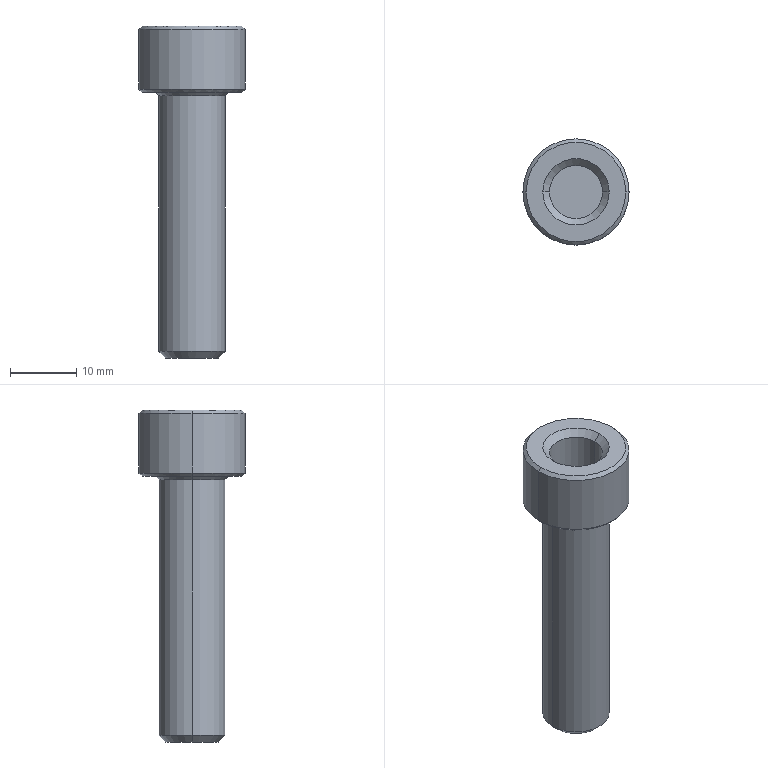Part | STEP file | fBY02F02M-00-11A | 1 solid | 20 faces | box 16 x 16 x 50 mm | volume 4764 mm3 | cone 10 | cylinder 6 | plane 4 | commonest cylinder face diameters 8 x2 10 x2 16 x2
STEP:
#1=CARTESIAN_POINT('',(0.,0.,0.));
#2=DIRECTION('',(0.,0.,1.));
#3=DIRECTION('',(1.,0.,0.));
#4=AXIS2_PLACEMENT_3D('',#1,#2,#3);
#5=CARTESIAN_POINT('',(-5.,0.,39.5));
#6=VERTEX_POINT('',#5);
#7=CARTESIAN_POINT('',(5.,0.,39.5));
#8=VERTEX_POINT('',#7);
#9=CARTESIAN_POINT('',(0.,0.,39.5));
#10=DIRECTION('',(0.,0.,-1.));
#11=DIRECTION('',(-1.,0.,0.));
#12=AXIS2_PLACEMENT_3D('',#9,#10,#11);
#13=CIRCLE('',#12,5.);
#14=CARTESIAN_POINT('',(0.,0.,40.));
#15=DIRECTION('',(0.,0.,-1.));
#16=DIRECTION('',(-1.,0.,0.));
#17=AXIS2_PLACEMENT_3D('',#14,#15,#16);
#18=CYLINDRICAL_SURFACE('',#17,5.);
#19=CARTESIAN_POINT('',(0.,0.5));
#20=DIRECTION('',(1.,0.));
#21=VECTOR('',#20,1.);
#22=LINE('',#19,#21);
#23=(GEOMETRIC_REPRESENTATION_CONTEXT(2)PARAMETRIC_REPRESENTATION_CONTEXT()REPRESENTATION_CONTEXT('',''));
#24=DEFINITIONAL_REPRESENTATION('',(#22),#23);
#25=PCURVE('',#18,#24);
#26=CARTESIAN_POINT('',(0.,0.,40.));
#27=DIRECTION('',(0.,0.,1.));
#28=DIRECTION('',(1.,0.,0.));
#29=AXIS2_PLACEMENT_3D('',#26,#27,#28);
#30=CONICAL_SURFACE('',#29,5.5,0.7854);
#31=CARTESIAN_POINT('',(3.142,-0.5));
#32=DIRECTION('',(-1.,0.));
#33=VECTOR('',#32,1.);
#34=LINE('',#31,#33);
#35=(GEOMETRIC_REPRESENTATION_CONTEXT(2)PARAMETRIC_REPRESENTATION_CONTEXT()REPRESENTATION_CONTEXT('',''));
#36=DEFINITIONAL_REPRESENTATION('',(#34),#35);
#37=PCURVE('',#30,#36);
#38=SURFACE_CURVE('',#13,(#25,#37),.PCURVE_S1.);
#39=EDGE_CURVE('',#6,#8,#38,.T.);
#40=ORIENTED_EDGE('',*,*,#39,.T.);
#41=CARTESIAN_POINT('',(5.,0.,1.));
#42=VERTEX_POINT('',#41);
#43=CARTESIAN_POINT('',(5.,0.,40.));
#44=DIRECTION('',(0.,0.,-1.));
#45=VECTOR('',#44,1.);
#46=LINE('',#43,#45);
#47=CARTESIAN_POINT('',(3.142,0.));
#48=DIRECTION('',(0.,1.));
#49=VECTOR('',#48,1.);
#50=LINE('',#47,#49);
#51=(GEOMETRIC_REPRESENTATION_CONTEXT(2)PARAMETRIC_REPRESENTATION_CONTEXT()REPRESENTATION_CONTEXT('',''));
#52=DEFINITIONAL_REPRESENTATION('',(#50),#51);
#53=PCURVE('',#18,#52);
#54=CARTESIAN_POINT('',(0.,0.,40.));
#55=DIRECTION('',(0.,0.,-1.));
#56=DIRECTION('',(-1.,0.,0.));
#57=AXIS2_PLACEMENT_3D('',#54,#55,#56);
#58=CYLINDRICAL_SURFACE('',#57,5.);
#59=CARTESIAN_POINT('',(3.142,0.));
#60=DIRECTION('',(0.,1.));
#61=VECTOR('',#60,1.);
#62=LINE('',#59,#61);
#63=(GEOMETRIC_REPRESENTATION_CONTEXT(2)PARAMETRIC_REPRESENTATION_CONTEXT()REPRESENTATION_CONTEXT('',''));
#64=DEFINITIONAL_REPRESENTATION('',(#62),#63);
#65=PCURVE('',#58,#64);
#66=SURFACE_CURVE('',#46,(#53,#65),.PCURVE_S1.);
#67=EDGE_CURVE('',#8,#42,#66,.T.);
#68=ORIENTED_EDGE('',*,*,#67,.T.);
#69=CARTESIAN_POINT('',(-5.,0.,1.));
#70=VERTEX_POINT('',#69);
#71=CARTESIAN_POINT('',(0.,0.,1.));
#72=DIRECTION('',(0.,0.,1.));
#73=DIRECTION('',(-1.,0.,0.));
#74=AXIS2_PLACEMENT_3D('',#71,#72,#73);
#75=CIRCLE('',#74,5.);
#76=CARTESIAN_POINT('',(6.283,39.));
#77=DIRECTION('',(-1.,0.));
#78=VECTOR('',#77,1.);
#79=LINE('',#76,#78);
#80=(GEOMETRIC_REPRESENTATION_CONTEXT(2)PARAMETRIC_REPRESENTATION_CONTEXT()REPRESENTATION_CONTEXT('',''));
#81=DEFINITIONAL_REPRESENTATION('',(#79),#80);
#82=PCURVE('',#18,#81);
#83=CARTESIAN_POINT('',(0.,0.,1.));
#84=DIRECTION('',(0.,0.,1.));
#85=DIRECTION('',(1.,0.,0.));
#86=AXIS2_PLACEMENT_3D('',#83,#84,#85);
#87=CONICAL_SURFACE('',#86,5.,0.7854);
#88=CARTESIAN_POINT('',(-3.142,0.));
#89=DIRECTION('',(1.,0.));
#90=VECTOR('',#89,1.);
#91=LINE('',#88,#90);
#92=(GEOMETRIC_REPRESENTATION_CONTEXT(2)PARAMETRIC_REPRESENTATION_CONTEXT()REPRESENTATION_CONTEXT('',''));
#93=DEFINITIONAL_REPRESENTATION('',(#91),#92);
#94=PCURVE('',#87,#93);
#95=SURFACE_CURVE('',#75,(#82,#94),.PCURVE_S1.);
#96=EDGE_CURVE('',#42,#70,#95,.T.);
#97=ORIENTED_EDGE('',*,*,#96,.T.);
#98=CARTESIAN_POINT('',(-5.,0.,40.));
#99=DIRECTION('',(0.,0.,-1.));
#100=VECTOR('',#99,1.);
#101=LINE('',#98,#100);
#102=CARTESIAN_POINT('',(0.,0.));
#103=DIRECTION('',(0.,1.));
#104=VECTOR('',#103,1.);
#105=LINE('',#102,#104);
#106=(GEOMETRIC_REPRESENTATION_CONTEXT(2)PARAMETRIC_REPRESENTATION_CONTEXT()REPRESENTATION_CONTEXT('',''));
#107=DEFINITIONAL_REPRESENTATION('',(#105),#106);
#108=PCURVE('',#18,#107);
#109=CARTESIAN_POINT('',(6.283,0.));
#110=DIRECTION('',(0.,1.));
#111=VECTOR('',#110,1.);
#112=LINE('',#109,#111);
#113=(GEOMETRIC_REPRESENTATION_CONTEXT(2)PARAMETRIC_REPRESENTATION_CONTEXT()REPRESENTATION_CONTEXT('',''));
#114=DEFINITIONAL_REPRESENTATION('',(#112),#113);
#115=PCURVE('',#58,#114);
#116=SURFACE_CURVE('',#101,(#108,#115),.PCURVE_S1.);
#117=EDGE_CURVE('',#6,#70,#116,.T.);
#118=ORIENTED_EDGE('',*,*,#117,.F.);
#119=EDGE_LOOP('',(#40,#68,#97,#118));
#120=FACE_BOUND('',#119,.T.);
#121=ADVANCED_FACE('',(#120),#18,.T.);
#122=CARTESIAN_POINT('',(4.,0.,0.));
#123=VERTEX_POINT('',#122);
#124=CARTESIAN_POINT('',(-4.,0.,0.));
#125=VERTEX_POINT('',#124);
#126=CARTESIAN_POINT('',(0.,0.,0.));
#127=DIRECTION('',(0.,0.,1.));
#128=DIRECTION('',(1.,0.,0.));
#129=AXIS2_PLACEMENT_3D('',#126,#127,#128);
#130=CIRCLE('',#129,4.);
#131=CARTESIAN_POINT('',(0.,-1.));
#132=DIRECTION('',(1.,0.));
#133=VECTOR('',#132,1.);
#134=LINE('',#131,#133);
#135=(GEOMETRIC_REPRESENTATION_CONTEXT(2)PARAMETRIC_REPRESENTATION_CONTEXT()REPRESENTATION_CONTEXT('',''));
#136=DEFINITIONAL_REPRESENTATION('',(#134),#135);
#137=PCURVE('',#87,#136);
#138=CARTESIAN_POINT('',(0.,0.,0.));
#139=DIRECTION('',(0.,0.,1.));
#140=DIRECTION('',(1.,0.,0.));
#141=AXIS2_PLACEMENT_3D('',#138,#139,#140);
#142=PLANE('',#141);
#143=CARTESIAN_POINT('',(0.,0.));
#144=DIRECTION('',(1.,0.));
#145=AXIS2_PLACEMENT_2D('',#143,#144);
#146=CIRCLE('',#145,4.);
#147=(GEOMETRIC_REPRESENTATION_CONTEXT(2)PARAMETRIC_REPRESENTATION_CONTEXT()REPRESENTATION_CONTEXT('',''));
#148=DEFINITIONAL_REPRESENTATION('',(#146),#147);
#149=PCURVE('',#142,#148);
#150=SURFACE_CURVE('',#130,(#137,#149),.PCURVE_S1.);
#151=EDGE_CURVE('',#123,#125,#150,.T.);
#152=ORIENTED_EDGE('',*,*,#151,.T.);
#153=CARTESIAN_POINT('',(-5.,0.,1.));
#154=DIRECTION('',(-0.7071,0.,0.7071));
#155=VECTOR('',#154,1.);
#156=LINE('',#153,#155);
#157=CARTESIAN_POINT('',(3.142,0.));
#158=DIRECTION('',(0.,1.));
#159=VECTOR('',#158,1.);
#160=LINE('',#157,#159);
#161=(GEOMETRIC_REPRESENTATION_CONTEXT(2)PARAMETRIC_REPRESENTATION_CONTEXT()REPRESENTATION_CONTEXT('',''));
#162=DEFINITIONAL_REPRESENTATION('',(#160),#161);
#163=PCURVE('',#87,#162);
#164=CARTESIAN_POINT('',(0.,0.,1.));
#165=DIRECTION('',(0.,0.,1.));
#166=DIRECTION('',(1.,0.,0.));
#167=AXIS2_PLACEMENT_3D('',#164,#165,#166);
#168=CONICAL_SURFACE('',#167,5.,0.7854);
#169=CARTESIAN_POINT('',(3.142,0.));
#170=DIRECTION('',(0.,1.));
#171=VECTOR('',#170,1.);
#172=LINE('',#169,#171);
#173=(GEOMETRIC_REPRESENTATION_CONTEXT(2)PARAMETRIC_REPRESENTATION_CONTEXT()REPRESENTATION_CONTEXT('',''));
#174=DEFINITIONAL_REPRESENTATION('',(#172),#173);
#175=PCURVE('',#168,#174);
#176=SURFACE_CURVE('',#156,(#163,#175),.PCURVE_S1.);
#177=EDGE_CURVE('',#125,#70,#176,.T.);
#178=ORIENTED_EDGE('',*,*,#177,.T.);
#179=ORIENTED_EDGE('',*,*,#96,.F.);
#180=CARTESIAN_POINT('',(5.,0.,1.));
#181=DIRECTION('',(0.7071,0.,0.7071));
#182=VECTOR('',#181,1.);
#183=LINE('',#180,#182);
#184=CARTESIAN_POINT('',(0.,0.));
#185=DIRECTION('',(0.,1.));
#186=VECTOR('',#185,1.);
#187=LINE('',#184,#186);
#188=(GEOMETRIC_REPRESENTATION_CONTEXT(2)PARAMETRIC_REPRESENTATION_CONTEXT()REPRESENTATION_CONTEXT('',''));
#189=DEFINITIONAL_REPRESENTATION('',(#187),#188);
#190=PCURVE('',#87,#189);
#191=CARTESIAN_POINT('',(6.283,0.));
#192=DIRECTION('',(0.,1.));
#193=VECTOR('',#192,1.);
#194=LINE('',#191,#193);
#195=(GEOMETRIC_REPRESENTATION_CONTEXT(2)PARAMETRIC_REPRESENTATION_CONTEXT()REPRESENTATION_CONTEXT('',''));
#196=DEFINITIONAL_REPRESENTATION('',(#194),#195);
#197=PCURVE('',#168,#196);
#198=SURFACE_CURVE('',#183,(#190,#197),.PCURVE_S1.);
#199=EDGE_CURVE('',#123,#42,#198,.T.);
#200=ORIENTED_EDGE('',*,*,#199,.F.);
#201=EDGE_LOOP('',(#152,#178,#179,#200));
#202=FACE_BOUND('',#201,.T.);
#203=ADVANCED_FACE('',(#202),#87,.T.);
#204=ORIENTED_EDGE('',*,*,#39,.F.);
#205=CARTESIAN_POINT('',(-5.5,0.,40.));
#206=VERTEX_POINT('',#205);
#207=CARTESIAN_POINT('',(-5.5,0.,40.));
#208=DIRECTION('',(-0.7071,0.,0.7071));
#209=VECTOR('',#208,1.);
#210=LINE('',#207,#209);
#211=CARTESIAN_POINT('',(3.142,0.));
#212=DIRECTION('',(0.,1.));
#213=VECTOR('',#212,1.);
#214=LINE('',#211,#213);
#215=(GEOMETRIC_REPRESENTATION_CONTEXT(2)PARAMETRIC_REPRESENTATION_CONTEXT()REPRESENTATION_CONTEXT('',''));
#216=DEFINITIONAL_REPRESENTATION('',(#214),#215);
#217=PCURVE('',#30,#216);
#218=CARTESIAN_POINT('',(0.,0.,40.));
#219=DIRECTION('',(0.,0.,1.));
#220=DIRECTION('',(1.,0.,0.));
#221=AXIS2_PLACEMENT_3D('',#218,#219,#220);
#222=CONICAL_SURFACE('',#221,5.5,0.7854);
#223=CARTESIAN_POINT('',(3.142,0.));
#224=DIRECTION('',(0.,1.));
#225=VECTOR('',#224,1.);
#226=LINE('',#223,#225);
#227=(GEOMETRIC_REPRESENTATION_CONTEXT(2)PARAMETRIC_REPRESENTATION_CONTEXT()REPRESENTATION_CONTEXT('',''));
#228=DEFINITIONAL_REPRESENTATION('',(#226),#227);
#229=PCURVE('',#222,#228);
#230=SURFACE_CURVE('',#210,(#217,#229),.PCURVE_S1.);
#231=EDGE_CURVE('',#6,#206,#230,.T.);
#232=ORIENTED_EDGE('',*,*,#231,.T.);
#233=CARTESIAN_POINT('',(5.5,0.,40.));
#234=VERTEX_POINT('',#233);
#235=CARTESIAN_POINT('',(0.,0.,40.));
#236=DIRECTION('',(0.,0.,-1.));
#237=DIRECTION('',(1.,0.,0.));
#238=AXIS2_PLACEMENT_3D('',#235,#236,#237);
#239=CIRCLE('',#238,5.5);
#240=CARTESIAN_POINT('',(6.283,0.));
#241=DIRECTION('',(-1.,0.));
#242=VECTOR('',#241,1.);
#243=LINE('',#240,#242);
#244=(GEOMETRIC_REPRESENTATION_CONTEXT(2)PARAMETRIC_REPRESENTATION_CONTEXT()REPRESENTATION_CONTEXT('',''));
#245=DEFINITIONAL_REPRESENTATION('',(#243),#244);
#246=PCURVE('',#30,#245);
#247=CARTESIAN_POINT('',(0.,0.,40.));
#248=DIRECTION('',(0.,0.,1.));
#249=DIRECTION('',(1.,0.,0.));
#250=AXIS2_PLACEMENT_3D('',#247,#248,#249);
#251=PLANE('',#250);
#252=CARTESIAN_POINT('',(5.5,0.));
#253=CARTESIAN_POINT('',(5.5,-9.526));
#254=CARTESIAN_POINT('',(-2.75,-4.763));
#255=CARTESIAN_POINT('',(-11.,0.));
#256=CARTESIAN_POINT('',(-2.75,4.763));
#257=CARTESIAN_POINT('',(5.5,9.526));
#258=CARTESIAN_POINT('',(5.5,0.));
#259=(BOUNDED_CURVE()B_SPLINE_CURVE(2,(#252,#253,#254,#255,#256,#257,#258),.UNSPECIFIED.,.T.,.F.)B_SPLINE_CURVE_WITH_KNOTS((1,2,2,2,2,1),(-2.094,0.,2.094,4.189,6.283,8.378),.UNSPECIFIED.)CURVE()GEOMETRIC_REPRESENTATION_ITEM()RATIONAL_B_SPLINE_CURVE((1.,0.5,1.,0.5,1.,0.5,1.))REPRESENTATION_ITEM(''));
#260=(GEOMETRIC_REPRESENTATION_CONTEXT(2)PARAMETRIC_REPRESENTATION_CONTEXT()REPRESENTATION_CONTEXT('',''));
#261=DEFINITIONAL_REPRESENTATION('',(#259),#260);
#262=PCURVE('',#251,#261);
#263=SURFACE_CURVE('',#239,(#246,#262),.PCURVE_S1.);
#264=EDGE_CURVE('',#206,#234,#263,.T.);
#265=ORIENTED_EDGE('',*,*,#264,.T.);
#266=CARTESIAN_POINT('',(5.5,0.,40.));
#267=DIRECTION('',(0.7071,0.,0.7071));
#268=VECTOR('',#267,1.);
#269=LINE('',#266,#268);
#270=CARTESIAN_POINT('',(0.,0.));
#271=DIRECTION('',(0.,1.));
#272=VECTOR('',#271,1.);
#273=LINE('',#270,#272);
#274=(GEOMETRIC_REPRESENTATION_CONTEXT(2)PARAMETRIC_REPRESENTATION_CONTEXT()REPRESENTATION_CONTEXT('',''));
#275=DEFINITIONAL_REPRESENTATION('',(#273),#274);
#276=PCURVE('',#30,#275);
#277=CARTESIAN_POINT('',(6.283,0.));
#278=DIRECTION('',(0.,1.));
#279=VECTOR('',#278,1.);
#280=LINE('',#277,#279);
#281=(GEOMETRIC_REPRESENTATION_CONTEXT(2)PARAMETRIC_REPRESENTATION_CONTEXT()REPRESENTATION_CONTEXT('',''));
#282=DEFINITIONAL_REPRESENTATION('',(#280),#281);
#283=PCURVE('',#222,#282);
#284=SURFACE_CURVE('',#269,(#276,#283),.PCURVE_S1.);
#285=EDGE_CURVE('',#8,#234,#284,.T.);
#286=ORIENTED_EDGE('',*,*,#285,.F.);
#287=EDGE_LOOP('',(#204,#232,#265,#286));
#288=FACE_BOUND('',#287,.T.);
#289=ADVANCED_FACE('',(#288),#30,.T.);
#290=CARTESIAN_POINT('',(7.5,0.,40.));
#291=VERTEX_POINT('',#290);
#292=CARTESIAN_POINT('',(-7.5,0.,40.));
#293=VERTEX_POINT('',#292);
#294=CARTESIAN_POINT('',(0.,0.,40.));
#295=DIRECTION('',(0.,0.,1.));
#296=DIRECTION('',(1.,0.,0.));
#297=AXIS2_PLACEMENT_3D('',#294,#295,#296);
#298=CIRCLE('',#297,7.5);
#299=CARTESIAN_POINT('',(0.,0.,40.5));
#300=DIRECTION('',(0.,0.,1.));
#301=DIRECTION('',(1.,0.,0.));
#302=AXIS2_PLACEMENT_3D('',#299,#300,#301);
#303=CONICAL_SURFACE('',#302,8.,0.7854);
#304=CARTESIAN_POINT('',(0.,-0.5));
#305=DIRECTION('',(1.,0.));
#306=VECTOR('',#305,1.);
#307=LINE('',#304,#306);
#308=(GEOMETRIC_REPRESENTATION_CONTEXT(2)PARAMETRIC_REPRESENTATION_CONTEXT()REPRESENTATION_CONTEXT('',''));
#309=DEFINITIONAL_REPRESENTATION('',(#307),#308);
#310=PCURVE('',#303,#309);
#311=CARTESIAN_POINT('',(0.,0.));
#312=DIRECTION('',(1.,0.));
#313=AXIS2_PLACEMENT_2D('',#311,#312);
#314=CIRCLE('',#313,7.5);
#315=(GEOMETRIC_REPRESENTATION_CONTEXT(2)PARAMETRIC_REPRESENTATION_CONTEXT()REPRESENTATION_CONTEXT('',''));
#316=DEFINITIONAL_REPRESENTATION('',(#314),#315);
#317=PCURVE('',#251,#316);
#318=SURFACE_CURVE('',#298,(#310,#317),.PCURVE_S1.);
#319=EDGE_CURVE('',#291,#293,#318,.T.);
#320=ORIENTED_EDGE('',*,*,#319,.T.);
#321=CARTESIAN_POINT('',(-8.,0.,40.5));
#322=VERTEX_POINT('',#321);
#323=CARTESIAN_POINT('',(-8.,0.,40.5));
#324=DIRECTION('',(-0.7071,0.,0.7071));
#325=VECTOR('',#324,1.);
#326=LINE('',#323,#325);
#327=CARTESIAN_POINT('',(3.142,0.));
#328=DIRECTION('',(0.,1.));
#329=VECTOR('',#328,1.);
#330=LINE('',#327,#329);
#331=(GEOMETRIC_REPRESENTATION_CONTEXT(2)PARAMETRIC_REPRESENTATION_CONTEXT()REPRESENTATION_CONTEXT('',''));
#332=DEFINITIONAL_REPRESENTATION('',(#330),#331);
#333=PCURVE('',#303,#332);
#334=CARTESIAN_POINT('',(0.,0.,40.5));
#335=DIRECTION('',(0.,0.,1.));
#336=DIRECTION('',(1.,0.,0.));
#337=AXIS2_PLACEMENT_3D('',#334,#335,#336);
#338=CONICAL_SURFACE('',#337,8.,0.7854);
#339=CARTESIAN_POINT('',(3.142,0.));
#340=DIRECTION('',(0.,1.));
#341=VECTOR('',#340,1.);
#342=LINE('',#339,#341);
#343=(GEOMETRIC_REPRESENTATION_CONTEXT(2)PARAMETRIC_REPRESENTATION_CONTEXT()REPRESENTATION_CONTEXT('',''));
#344=DEFINITIONAL_REPRESENTATION('',(#342),#343);
#345=PCURVE('',#338,#344);
#346=SURFACE_CURVE('',#326,(#333,#345),.PCURVE_S1.);
#347=EDGE_CURVE('',#293,#322,#346,.T.);
#348=ORIENTED_EDGE('',*,*,#347,.T.);
#349=CARTESIAN_POINT('',(8.,0.,40.5));
#350=VERTEX_POINT('',#349);
#351=CARTESIAN_POINT('',(0.,0.,40.5));
#352=DIRECTION('',(0.,0.,-1.));
#353=DIRECTION('',(1.,0.,0.));
#354=AXIS2_PLACEMENT_3D('',#351,#352,#353);
#355=CIRCLE('',#354,8.);
#356=CARTESIAN_POINT('',(6.283,0.));
#357=DIRECTION('',(-1.,0.));
#358=VECTOR('',#357,1.);
#359=LINE('',#356,#358);
#360=(GEOMETRIC_REPRESENTATION_CONTEXT(2)PARAMETRIC_REPRESENTATION_CONTEXT()REPRESENTATION_CONTEXT('',''));
#361=DEFINITIONAL_REPRESENTATION('',(#359),#360);
#362=PCURVE('',#303,#361);
#363=CARTESIAN_POINT('',(0.,0.,50.));
#364=DIRECTION('',(0.,0.,-1.));
#365=DIRECTION('',(-1.,0.,0.));
#366=AXIS2_PLACEMENT_3D('',#363,#364,#365);
#367=CYLINDRICAL_SURFACE('',#366,8.);
#368=CARTESIAN_POINT('',(-3.142,9.5));
#369=DIRECTION('',(1.,0.));
#370=VECTOR('',#369,1.);
#371=LINE('',#368,#370);
#372=(GEOMETRIC_REPRESENTATION_CONTEXT(2)PARAMETRIC_REPRESENTATION_CONTEXT()REPRESENTATION_CONTEXT('',''));
#373=DEFINITIONAL_REPRESENTATION('',(#371),#372);
#374=PCURVE('',#367,#373);
#375=SURFACE_CURVE('',#355,(#362,#374),.PCURVE_S1.);
#376=EDGE_CURVE('',#322,#350,#375,.T.);
#377=ORIENTED_EDGE('',*,*,#376,.T.);
#378=CARTESIAN_POINT('',(8.,0.,40.5));
#379=DIRECTION('',(0.7071,0.,0.7071));
#380=VECTOR('',#379,1.);
#381=LINE('',#378,#380);
#382=CARTESIAN_POINT('',(0.,0.));
#383=DIRECTION('',(0.,1.));
#384=VECTOR('',#383,1.);
#385=LINE('',#382,#384);
#386=(GEOMETRIC_REPRESENTATION_CONTEXT(2)PARAMETRIC_REPRESENTATION_CONTEXT()REPRESENTATION_CONTEXT('',''));
#387=DEFINITIONAL_REPRESENTATION('',(#385),#386);
#388=PCURVE('',#303,#387);
#389=CARTESIAN_POINT('',(6.283,0.));
#390=DIRECTION('',(0.,1.));
#391=VECTOR('',#390,1.);
#392=LINE('',#389,#391);
#393=(GEOMETRIC_REPRESENTATION_CONTEXT(2)PARAMETRIC_REPRESENTATION_CONTEXT()REPRESENTATION_CONTEXT('',''));
#394=DEFINITIONAL_REPRESENTATION('',(#392),#393);
#395=PCURVE('',#338,#394);
#396=SURFACE_CURVE('',#381,(#388,#395),.PCURVE_S1.);
#397=EDGE_CURVE('',#291,#350,#396,.T.);
#398=ORIENTED_EDGE('',*,*,#397,.F.);
#399=EDGE_LOOP('',(#320,#348,#377,#398));
#400=FACE_BOUND('',#399,.T.);
#401=ADVANCED_FACE('',(#400),#303,.T.);
#402=CARTESIAN_POINT('',(-8.,0.,49.5));
#403=VERTEX_POINT('',#402);
#404=CARTESIAN_POINT('',(8.,0.,49.5));
#405=VERTEX_POINT('',#404);
#406=CARTESIAN_POINT('',(0.,0.,49.5));
#407=DIRECTION('',(0.,0.,-1.));
#408=DIRECTION('',(-1.,0.,0.));
#409=AXIS2_PLACEMENT_3D('',#406,#407,#408);
#410=CIRCLE('',#409,8.);
#411=CARTESIAN_POINT('',(0.,0.5));
#412=DIRECTION('',(1.,0.));
#413=VECTOR('',#412,1.);
#414=LINE('',#411,#413);
#415=(GEOMETRIC_REPRESENTATION_CONTEXT(2)PARAMETRIC_REPRESENTATION_CONTEXT()REPRESENTATION_CONTEXT('',''));
#416=DEFINITIONAL_REPRESENTATION('',(#414),#415);
#417=PCURVE('',#367,#416);
#418=CARTESIAN_POINT('',(0.,0.,49.5));
#419=DIRECTION('',(0.,0.,-1.));
#420=DIRECTION('',(-1.,0.,0.));
#421=AXIS2_PLACEMENT_3D('',#418,#419,#420);
#422=CONICAL_SURFACE('',#421,8.,0.7854);
#423=CARTESIAN_POINT('',(0.,0.));
#424=DIRECTION('',(1.,0.));
#425=VECTOR('',#424,1.);
#426=LINE('',#423,#425);
#427=(GEOMETRIC_REPRESENTATION_CONTEXT(2)PARAMETRIC_REPRESENTATION_CONTEXT()REPRESENTATION_CONTEXT('',''));
#428=DEFINITIONAL_REPRESENTATION('',(#426),#427);
#429=PCURVE('',#422,#428);
#430=SURFACE_CURVE('',#410,(#417,#429),.PCURVE_S1.);
#431=EDGE_CURVE('',#403,#405,#430,.T.);
#432=ORIENTED_EDGE('',*,*,#431,.T.);
#433=CARTESIAN_POINT('',(8.,0.,50.));
#434=DIRECTION('',(0.,0.,-1.));
#435=VECTOR('',#434,1.);
#436=LINE('',#433,#435);
#437=CARTESIAN_POINT('',(3.142,0.));
#438=DIRECTION('',(0.,1.));
#439=VECTOR('',#438,1.);
#440=LINE('',#437,#439);
#441=(GEOMETRIC_REPRESENTATION_CONTEXT(2)PARAMETRIC_REPRESENTATION_CONTEXT()REPRESENTATION_CONTEXT('',''));
#442=DEFINITIONAL_REPRESENTATION('',(#440),#441);
#443=PCURVE('',#367,#442);
#444=CARTESIAN_POINT('',(0.,0.,50.));
#445=DIRECTION('',(0.,0.,-1.));
#446=DIRECTION('',(-1.,0.,0.));
#447=AXIS2_PLACEMENT_3D('',#444,#445,#446);
#448=CYLINDRICAL_SURFACE('',#447,8.);
#449=CARTESIAN_POINT('',(3.142,0.));
#450=DIRECTION('',(0.,1.));
#451=VECTOR('',#450,1.);
#452=LINE('',#449,#451);
#453=(GEOMETRIC_REPRESENTATION_CONTEXT(2)PARAMETRIC_REPRESENTATION_CONTEXT()REPRESENTATION_CONTEXT('',''));
#454=DEFINITIONAL_REPRESENTATION('',(#452),#453);
#455=PCURVE('',#448,#454);
#456=SURFACE_CURVE('',#436,(#443,#455),.PCURVE_S1.);
#457=EDGE_CURVE('',#405,#350,#456,.T.);
#458=ORIENTED_EDGE('',*,*,#457,.T.);
#459=ORIENTED_EDGE('',*,*,#376,.F.);
#460=CARTESIAN_POINT('',(-8.,0.,50.));
#461=DIRECTION('',(0.,0.,-1.));
#462=VECTOR('',#461,1.);
#463=LINE('',#460,#462);
#464=CARTESIAN_POINT('',(0.,0.));
#465=DIRECTION('',(0.,1.));
#466=VECTOR('',#465,1.);
#467=LINE('',#464,#466);
#468=(GEOMETRIC_REPRESENTATION_CONTEXT(2)PARAMETRIC_REPRESENTATION_CONTEXT()REPRESENTATION_CONTEXT('',''));
#469=DEFINITIONAL_REPRESENTATION('',(#467),#468);
#470=PCURVE('',#367,#469);
#471=CARTESIAN_POINT('',(6.283,0.));
#472=DIRECTION('',(0.,1.));
#473=VECTOR('',#472,1.);
#474=LINE('',#471,#473);
#475=(GEOMETRIC_REPRESENTATION_CONTEXT(2)PARAMETRIC_REPRESENTATION_CONTEXT()REPRESENTATION_CONTEXT('',''));
#476=DEFINITIONAL_REPRESENTATION('',(#474),#475);
#477=PCURVE('',#448,#476);
#478=SURFACE_CURVE('',#463,(#470,#477),.PCURVE_S1.);
#479=EDGE_CURVE('',#403,#322,#478,.T.);
#480=ORIENTED_EDGE('',*,*,#479,.F.);
#481=EDGE_LOOP('',(#432,#458,#459,#480));
#482=FACE_BOUND('',#481,.T.);
#483=ADVANCED_FACE('',(#482),#367,.T.);
#484=CARTESIAN_POINT('',(-7.5,0.,50.));
#485=VERTEX_POINT('',#484);
#486=CARTESIAN_POINT('',(7.5,0.,50.));
#487=VERTEX_POINT('',#486);
#488=CARTESIAN_POINT('',(0.,0.,50.));
#489=DIRECTION('',(0.,0.,-1.));
#490=DIRECTION('',(-1.,0.,0.));
#491=AXIS2_PLACEMENT_3D('',#488,#489,#490);
#492=CIRCLE('',#491,7.5);
#493=CARTESIAN_POINT('',(0.,-0.5));
#494=DIRECTION('',(1.,0.));
#495=VECTOR('',#494,1.);
#496=LINE('',#493,#495);
#497=(GEOMETRIC_REPRESENTATION_CONTEXT(2)PARAMETRIC_REPRESENTATION_CONTEXT()REPRESENTATION_CONTEXT('',''));
#498=DEFINITIONAL_REPRESENTATION('',(#496),#497);
#499=PCURVE('',#422,#498);
#500=CARTESIAN_POINT('',(0.,0.,50.));
#501=DIRECTION('',(0.,0.,1.));
#502=DIRECTION('',(1.,0.,0.));
#503=AXIS2_PLACEMENT_3D('',#500,#501,#502);
#504=PLANE('',#503);
#505=CARTESIAN_POINT('',(-7.5,0.));
#506=CARTESIAN_POINT('',(-7.5,12.99));
#507=CARTESIAN_POINT('',(3.75,6.495));
#508=CARTESIAN_POINT('',(15.,0.));
#509=CARTESIAN_POINT('',(3.75,-6.495));
#510=CARTESIAN_POINT('',(-7.5,-12.99));
#511=CARTESIAN_POINT('',(-7.5,0.));
#512=(BOUNDED_CURVE()B_SPLINE_CURVE(2,(#505,#506,#507,#508,#509,#510,#511),.UNSPECIFIED.,.T.,.F.)B_SPLINE_CURVE_WITH_KNOTS((1,2,2,2,2,1),(-2.094,0.,2.094,4.189,6.283,8.378),.UNSPECIFIED.)CURVE()GEOMETRIC_REPRESENTATION_ITEM()RATIONAL_B_SPLINE_CURVE((1.,0.5,1.,0.5,1.,0.5,1.))REPRESENTATION_ITEM(''));
#513=(GEOMETRIC_REPRESENTATION_CONTEXT(2)PARAMETRIC_REPRESENTATION_CONTEXT()REPRESENTATION_CONTEXT('',''));
#514=DEFINITIONAL_REPRESENTATION('',(#512),#513);
#515=PCURVE('',#504,#514);
#516=SURFACE_CURVE('',#492,(#499,#515),.PCURVE_S1.);
#517=EDGE_CURVE('',#485,#487,#516,.T.);
#518=ORIENTED_EDGE('',*,*,#517,.T.);
#519=CARTESIAN_POINT('',(8.,0.,49.5));
#520=DIRECTION('',(0.7071,0.,-0.7071));
#521=VECTOR('',#520,1.);
#522=LINE('',#519,#521);
#523=CARTESIAN_POINT('',(3.142,0.));
#524=DIRECTION('',(0.,1.));
#525=VECTOR('',#524,1.);
#526=LINE('',#523,#525);
#527=(GEOMETRIC_REPRESENTATION_CONTEXT(2)PARAMETRIC_REPRESENTATION_CONTEXT()REPRESENTATION_CONTEXT('',''));
#528=DEFINITIONAL_REPRESENTATION('',(#526),#527);
#529=PCURVE('',#422,#528);
#530=CARTESIAN_POINT('',(0.,0.,49.5));
#531=DIRECTION('',(0.,0.,-1.));
#532=DIRECTION('',(-1.,0.,0.));
#533=AXIS2_PLACEMENT_3D('',#530,#531,#532);
#534=CONICAL_SURFACE('',#533,8.,0.7854);
#535=CARTESIAN_POINT('',(3.142,0.));
#536=DIRECTION('',(0.,1.));
#537=VECTOR('',#536,1.);
#538=LINE('',#535,#537);
#539=(GEOMETRIC_REPRESENTATION_CONTEXT(2)PARAMETRIC_REPRESENTATION_CONTEXT()REPRESENTATION_CONTEXT('',''));
#540=DEFINITIONAL_REPRESENTATION('',(#538),#539);
#541=PCURVE('',#534,#540);
#542=SURFACE_CURVE('',#522,(#529,#541),.PCURVE_S1.);
#543=EDGE_CURVE('',#487,#405,#542,.T.);
#544=ORIENTED_EDGE('',*,*,#543,.T.);
#545=ORIENTED_EDGE('',*,*,#431,.F.);
#546=CARTESIAN_POINT('',(-8.,0.,49.5));
#547=DIRECTION('',(-0.7071,0.,-0.7071));
#548=VECTOR('',#547,1.);
#549=LINE('',#546,#548);
#550=CARTESIAN_POINT('',(0.,0.));
#551=DIRECTION('',(0.,1.));
#552=VECTOR('',#551,1.);
#553=LINE('',#550,#552);
#554=(GEOMETRIC_REPRESENTATION_CONTEXT(2)PARAMETRIC_REPRESENTATION_CONTEXT()REPRESENTATION_CONTEXT('',''));
#555=DEFINITIONAL_REPRESENTATION('',(#553),#554);
#556=PCURVE('',#422,#555);
#557=CARTESIAN_POINT('',(6.283,0.));
#558=DIRECTION('',(0.,1.));
#559=VECTOR('',#558,1.);
#560=LINE('',#557,#559);
#561=(GEOMETRIC_REPRESENTATION_CONTEXT(2)PARAMETRIC_REPRESENTATION_CONTEXT()REPRESENTATION_CONTEXT('',''));
#562=DEFINITIONAL_REPRESENTATION('',(#560),#561);
#563=PCURVE('',#534,#562);
#564=SURFACE_CURVE('',#549,(#556,#563),.PCURVE_S1.);
#565=EDGE_CURVE('',#485,#403,#564,.T.);
#566=ORIENTED_EDGE('',*,*,#565,.F.);
#567=EDGE_LOOP('',(#518,#544,#545,#566));
#568=FACE_BOUND('',#567,.T.);
#569=ADVANCED_FACE('',(#568),#422,.T.);
#570=CARTESIAN_POINT('',(4.,0.,49.));
#571=VERTEX_POINT('',#570);
#572=CARTESIAN_POINT('',(5.,0.,50.));
#573=VERTEX_POINT('',#572);
#574=CARTESIAN_POINT('',(5.,0.,50.));
#575=DIRECTION('',(0.7071,0.,0.7071));
#576=VECTOR('',#575,1.);
#577=LINE('',#574,#576);
#578=CARTESIAN_POINT('',(0.,0.,50.));
#579=DIRECTION('',(0.,0.,1.));
#580=DIRECTION('',(1.,0.,0.));
#581=AXIS2_PLACEMENT_3D('',#578,#579,#580);
#582=CONICAL_SURFACE('',#581,5.,0.7854);
#583=CARTESIAN_POINT('',(6.283,0.));
#584=DIRECTION('',(0.,1.));
#585=VECTOR('',#584,1.);
#586=LINE('',#583,#585);
#587=(GEOMETRIC_REPRESENTATION_CONTEXT(2)PARAMETRIC_REPRESENTATION_CONTEXT()REPRESENTATION_CONTEXT('',''));
#588=DEFINITIONAL_REPRESENTATION('',(#586),#587);
#589=PCURVE('',#582,#588);
#590=CARTESIAN_POINT('',(0.,0.,50.));
#591=DIRECTION('',(0.,0.,1.));
#592=DIRECTION('',(1.,0.,0.));
#593=AXIS2_PLACEMENT_3D('',#590,#591,#592);
#594=CONICAL_SURFACE('',#593,5.,0.7854);
#595=CARTESIAN_POINT('',(0.,0.));
#596=DIRECTION('',(0.,1.));
#597=VECTOR('',#596,1.);
#598=LINE('',#595,#597);
#599=(GEOMETRIC_REPRESENTATION_CONTEXT(2)PARAMETRIC_REPRESENTATION_CONTEXT()REPRESENTATION_CONTEXT('',''));
#600=DEFINITIONAL_REPRESENTATION('',(#598),#599);
#601=PCURVE('',#594,#600);
#602=SURFACE_CURVE('',#577,(#589,#601),.PCURVE_S1.);
#603=EDGE_CURVE('',#571,#573,#602,.T.);
#604=ORIENTED_EDGE('',*,*,#603,.T.);
#605=CARTESIAN_POINT('',(-5.,0.,50.));
#606=VERTEX_POINT('',#605);
#607=CARTESIAN_POINT('',(0.,0.,50.));
#608=DIRECTION('',(0.,0.,-1.));
#609=DIRECTION('',(1.,0.,0.));
#610=AXIS2_PLACEMENT_3D('',#607,#608,#609);
#611=CIRCLE('',#610,5.);
#612=CARTESIAN_POINT('',(6.283,0.));
#613=DIRECTION('',(-1.,0.));
#614=VECTOR('',#613,1.);
#615=LINE('',#612,#614);
#616=(GEOMETRIC_REPRESENTATION_CONTEXT(2)PARAMETRIC_REPRESENTATION_CONTEXT()REPRESENTATION_CONTEXT('',''));
#617=DEFINITIONAL_REPRESENTATION('',(#615),#616);
#618=PCURVE('',#582,#617);
#619=CARTESIAN_POINT('',(5.,0.));
#620=CARTESIAN_POINT('',(5.,-8.66));
#621=CARTESIAN_POINT('',(-2.5,-4.33));
#622=CARTESIAN_POINT('',(-10.,0.));
#623=CARTESIAN_POINT('',(-2.5,4.33));
#624=CARTESIAN_POINT('',(5.,8.66));
#625=CARTESIAN_POINT('',(5.,0.));
#626=(BOUNDED_CURVE()B_SPLINE_CURVE(2,(#619,#620,#621,#622,#623,#624,#625),.UNSPECIFIED.,.T.,.F.)B_SPLINE_CURVE_WITH_KNOTS((1,2,2,2,2,1),(-2.094,0.,2.094,4.189,6.283,8.378),.UNSPECIFIED.)CURVE()GEOMETRIC_REPRESENTATION_ITEM()RATIONAL_B_SPLINE_CURVE((1.,0.5,1.,0.5,1.,0.5,1.))REPRESENTATION_ITEM(''));
#627=(GEOMETRIC_REPRESENTATION_CONTEXT(2)PARAMETRIC_REPRESENTATION_CONTEXT()REPRESENTATION_CONTEXT('',''));
#628=DEFINITIONAL_REPRESENTATION('',(#626),#627);
#629=PCURVE('',#504,#628);
#630=SURFACE_CURVE('',#611,(#618,#629),.PCURVE_S1.);
#631=EDGE_CURVE('',#573,#606,#630,.T.);
#632=ORIENTED_EDGE('',*,*,#631,.T.);
#633=CARTESIAN_POINT('',(-4.,0.,49.));
#634=VERTEX_POINT('',#633);
#635=CARTESIAN_POINT('',(-5.,0.,50.));
#636=DIRECTION('',(-0.7071,0.,0.7071));
#637=VECTOR('',#636,1.);
#638=LINE('',#635,#637);
#639=CARTESIAN_POINT('',(3.142,0.));
#640=DIRECTION('',(0.,1.));
#641=VECTOR('',#640,1.);
#642=LINE('',#639,#641);
#643=(GEOMETRIC_REPRESENTATION_CONTEXT(2)PARAMETRIC_REPRESENTATION_CONTEXT()REPRESENTATION_CONTEXT('',''));
#644=DEFINITIONAL_REPRESENTATION('',(#642),#643);
#645=PCURVE('',#582,#644);
#646=CARTESIAN_POINT('',(3.142,0.));
#647=DIRECTION('',(0.,1.));
#648=VECTOR('',#647,1.);
#649=LINE('',#646,#648);
#650=(GEOMETRIC_REPRESENTATION_CONTEXT(2)PARAMETRIC_REPRESENTATION_CONTEXT()REPRESENTATION_CONTEXT('',''));
#651=DEFINITIONAL_REPRESENTATION('',(#649),#650);
#652=PCURVE('',#594,#651);
#653=SURFACE_CURVE('',#638,(#645,#652),.PCURVE_S1.);
#654=EDGE_CURVE('',#634,#606,#653,.T.);
#655=ORIENTED_EDGE('',*,*,#654,.F.);
#656=CARTESIAN_POINT('',(0.,0.,49.));
#657=DIRECTION('',(0.,0.,1.));
#658=DIRECTION('',(1.,0.,0.));
#659=AXIS2_PLACEMENT_3D('',#656,#657,#658);
#660=CIRCLE('',#659,4.);
#661=CARTESIAN_POINT('',(0.,-1.));
#662=DIRECTION('',(1.,0.));
#663=VECTOR('',#662,1.);
#664=LINE('',#661,#663);
#665=(GEOMETRIC_REPRESENTATION_CONTEXT(2)PARAMETRIC_REPRESENTATION_CONTEXT()REPRESENTATION_CONTEXT('',''));
#666=DEFINITIONAL_REPRESENTATION('',(#664),#665);
#667=PCURVE('',#582,#666);
#668=CARTESIAN_POINT('',(0.,0.,43.));
#669=DIRECTION('',(0.,0.,1.));
#670=DIRECTION('',(1.,0.,0.));
#671=AXIS2_PLACEMENT_3D('',#668,#669,#670);
#672=CYLINDRICAL_SURFACE('',#671,4.);
#673=CARTESIAN_POINT('',(0.,6.));
#674=DIRECTION('',(1.,0.));
#675=VECTOR('',#674,1.);
#676=LINE('',#673,#675);
#677=(GEOMETRIC_REPRESENTATION_CONTEXT(2)PARAMETRIC_REPRESENTATION_CONTEXT()REPRESENTATION_CONTEXT('',''));
#678=DEFINITIONAL_REPRESENTATION('',(#676),#677);
#679=PCURVE('',#672,#678);
#680=SURFACE_CURVE('',#660,(#667,#679),.PCURVE_S1.);
#681=EDGE_CURVE('',#634,#571,#680,.T.);
#682=ORIENTED_EDGE('',*,*,#681,.T.);
#683=EDGE_LOOP('',(#604,#632,#655,#682));
#684=FACE_BOUND('',#683,.F.);
#685=ADVANCED_FACE('',(#684),#582,.F.);
#686=CARTESIAN_POINT('',(4.,0.,43.));
#687=VERTEX_POINT('',#686);
#688=CARTESIAN_POINT('',(4.,0.,43.));
#689=DIRECTION('',(0.,0.,1.));
#690=VECTOR('',#689,1.);
#691=LINE('',#688,#690);
#692=CARTESIAN_POINT('',(6.283,0.));
#693=DIRECTION('',(0.,1.));
#694=VECTOR('',#693,1.);
#695=LINE('',#692,#694);
#696=(GEOMETRIC_REPRESENTATION_CONTEXT(2)PARAMETRIC_REPRESENTATION_CONTEXT()REPRESENTATION_CONTEXT('',''));
#697=DEFINITIONAL_REPRESENTATION('',(#695),#696);
#698=PCURVE('',#672,#697);
#699=CARTESIAN_POINT('',(0.,0.,43.));
#700=DIRECTION('',(0.,0.,1.));
#701=DIRECTION('',(1.,0.,0.));
#702=AXIS2_PLACEMENT_3D('',#699,#700,#701);
#703=CYLINDRICAL_SURFACE('',#702,4.);
#704=CARTESIAN_POINT('',(0.,0.));
#705=DIRECTION('',(0.,1.));
#706=VECTOR('',#705,1.);
#707=LINE('',#704,#706);
#708=(GEOMETRIC_REPRESENTATION_CONTEXT(2)PARAMETRIC_REPRESENTATION_CONTEXT()REPRESENTATION_CONTEXT('',''));
#709=DEFINITIONAL_REPRESENTATION('',(#707),#708);
#710=PCURVE('',#703,#709);
#711=SURFACE_CURVE('',#691,(#698,#710),.PCURVE_S1.);
#712=EDGE_CURVE('',#687,#571,#711,.T.);
#713=ORIENTED_EDGE('',*,*,#712,.T.);
#714=ORIENTED_EDGE('',*,*,#681,.F.);
#715=CARTESIAN_POINT('',(-4.,0.,43.));
#716=VERTEX_POINT('',#715);
#717=CARTESIAN_POINT('',(-4.,0.,43.));
#718=DIRECTION('',(0.,0.,1.));
#719=VECTOR('',#718,1.);
#720=LINE('',#717,#719);
#721=CARTESIAN_POINT('',(3.142,0.));
#722=DIRECTION('',(0.,1.));
#723=VECTOR('',#722,1.);
#724=LINE('',#721,#723);
#725=(GEOMETRIC_REPRESENTATION_CONTEXT(2)PARAMETRIC_REPRESENTATION_CONTEXT()REPRESENTATION_CONTEXT('',''));
#726=DEFINITIONAL_REPRESENTATION('',(#724),#725);
#727=PCURVE('',#672,#726);
#728=CARTESIAN_POINT('',(3.142,0.));
#729=DIRECTION('',(0.,1.));
#730=VECTOR('',#729,1.);
#731=LINE('',#728,#730);
#732=(GEOMETRIC_REPRESENTATION_CONTEXT(2)PARAMETRIC_REPRESENTATION_CONTEXT()REPRESENTATION_CONTEXT('',''));
#733=DEFINITIONAL_REPRESENTATION('',(#731),#732);
#734=PCURVE('',#703,#733);
#735=SURFACE_CURVE('',#720,(#727,#734),.PCURVE_S1.);
#736=EDGE_CURVE('',#716,#634,#735,.T.);
#737=ORIENTED_EDGE('',*,*,#736,.F.);
#738=CARTESIAN_POINT('',(0.,0.,43.));
#739=DIRECTION('',(0.,0.,1.));
#740=DIRECTION('',(1.,0.,0.));
#741=AXIS2_PLACEMENT_3D('',#738,#739,#740);
#742=CIRCLE('',#741,4.);
#743=CARTESIAN_POINT('',(0.,0.));
#744=DIRECTION('',(1.,0.));
#745=VECTOR('',#744,1.);
#746=LINE('',#743,#745);
#747=(GEOMETRIC_REPRESENTATION_CONTEXT(2)PARAMETRIC_REPRESENTATION_CONTEXT()REPRESENTATION_CONTEXT('',''));
#748=DEFINITIONAL_REPRESENTATION('',(#746),#747);
#749=PCURVE('',#672,#748);
#750=CARTESIAN_POINT('',(0.,0.,43.));
#751=DIRECTION('',(0.,0.,1.));
#752=DIRECTION('',(1.,0.,0.));
#753=AXIS2_PLACEMENT_3D('',#750,#751,#752);
#754=PLANE('',#753);
#755=CARTESIAN_POINT('',(0.,0.));
#756=DIRECTION('',(1.,0.));
#757=AXIS2_PLACEMENT_2D('',#755,#756);
#758=CIRCLE('',#757,4.);
#759=(GEOMETRIC_REPRESENTATION_CONTEXT(2)PARAMETRIC_REPRESENTATION_CONTEXT()REPRESENTATION_CONTEXT('',''));
#760=DEFINITIONAL_REPRESENTATION('',(#758),#759);
#761=PCURVE('',#754,#760);
#762=SURFACE_CURVE('',#742,(#749,#761),.PCURVE_S1.);
#763=EDGE_CURVE('',#716,#687,#762,.T.);
#764=ORIENTED_EDGE('',*,*,#763,.T.);
#765=EDGE_LOOP('',(#713,#714,#737,#764));
#766=FACE_BOUND('',#765,.F.);
#767=ADVANCED_FACE('',(#766),#672,.F.);
#768=ORIENTED_EDGE('',*,*,#67,.F.);
#769=CARTESIAN_POINT('',(0.,0.,39.5));
#770=DIRECTION('',(0.,0.,-1.));
#771=DIRECTION('',(-1.,0.,0.));
#772=AXIS2_PLACEMENT_3D('',#769,#770,#771);
#773=CIRCLE('',#772,5.);
#774=CARTESIAN_POINT('',(0.,0.5));
#775=DIRECTION('',(1.,0.));
#776=VECTOR('',#775,1.);
#777=LINE('',#774,#776);
#778=(GEOMETRIC_REPRESENTATION_CONTEXT(2)PARAMETRIC_REPRESENTATION_CONTEXT()REPRESENTATION_CONTEXT('',''));
#779=DEFINITIONAL_REPRESENTATION('',(#777),#778);
#780=PCURVE('',#58,#779);
#781=CARTESIAN_POINT('',(9.425,-0.5));
#782=DIRECTION('',(-1.,0.));
#783=VECTOR('',#782,1.);
#784=LINE('',#781,#783);
#785=(GEOMETRIC_REPRESENTATION_CONTEXT(2)PARAMETRIC_REPRESENTATION_CONTEXT()REPRESENTATION_CONTEXT('',''));
#786=DEFINITIONAL_REPRESENTATION('',(#784),#785);
#787=PCURVE('',#222,#786);
#788=SURFACE_CURVE('',#773,(#780,#787),.PCURVE_S1.);
#789=EDGE_CURVE('',#8,#6,#788,.T.);
#790=ORIENTED_EDGE('',*,*,#789,.T.);
#791=ORIENTED_EDGE('',*,*,#117,.T.);
#792=CARTESIAN_POINT('',(0.,0.,1.));
#793=DIRECTION('',(0.,0.,1.));
#794=DIRECTION('',(-1.,0.,0.));
#795=AXIS2_PLACEMENT_3D('',#792,#793,#794);
#796=CIRCLE('',#795,5.);
#797=CARTESIAN_POINT('',(6.283,39.));
#798=DIRECTION('',(-1.,0.));
#799=VECTOR('',#798,1.);
#800=LINE('',#797,#799);
#801=(GEOMETRIC_REPRESENTATION_CONTEXT(2)PARAMETRIC_REPRESENTATION_CONTEXT()REPRESENTATION_CONTEXT('',''));
#802=DEFINITIONAL_REPRESENTATION('',(#800),#801);
#803=PCURVE('',#58,#802);
#804=CARTESIAN_POINT('',(3.142,0.));
#805=DIRECTION('',(1.,0.));
#806=VECTOR('',#805,1.);
#807=LINE('',#804,#806);
#808=(GEOMETRIC_REPRESENTATION_CONTEXT(2)PARAMETRIC_REPRESENTATION_CONTEXT()REPRESENTATION_CONTEXT('',''));
#809=DEFINITIONAL_REPRESENTATION('',(#807),#808);
#810=PCURVE('',#168,#809);
#811=SURFACE_CURVE('',#796,(#803,#810),.PCURVE_S1.);
#812=EDGE_CURVE('',#70,#42,#811,.T.);
#813=ORIENTED_EDGE('',*,*,#812,.T.);
#814=EDGE_LOOP('',(#768,#790,#791,#813));
#815=FACE_BOUND('',#814,.T.);
#816=ADVANCED_FACE('',(#815),#58,.T.);
#817=ORIENTED_EDGE('',*,*,#177,.F.);
#818=CARTESIAN_POINT('',(0.,0.,0.));
#819=DIRECTION('',(0.,0.,1.));
#820=DIRECTION('',(1.,0.,0.));
#821=AXIS2_PLACEMENT_3D('',#818,#819,#820);
#822=CIRCLE('',#821,4.);
#823=CARTESIAN_POINT('',(0.,-1.));
#824=DIRECTION('',(1.,0.));
#825=VECTOR('',#824,1.);
#826=LINE('',#823,#825);
#827=(GEOMETRIC_REPRESENTATION_CONTEXT(2)PARAMETRIC_REPRESENTATION_CONTEXT()REPRESENTATION_CONTEXT('',''));
#828=DEFINITIONAL_REPRESENTATION('',(#826),#827);
#829=PCURVE('',#168,#828);
#830=CARTESIAN_POINT('',(0.,0.));
#831=DIRECTION('',(1.,0.));
#832=AXIS2_PLACEMENT_2D('',#830,#831);
#833=CIRCLE('',#832,4.);
#834=(GEOMETRIC_REPRESENTATION_CONTEXT(2)PARAMETRIC_REPRESENTATION_CONTEXT()REPRESENTATION_CONTEXT('',''));
#835=DEFINITIONAL_REPRESENTATION('',(#833),#834);
#836=PCURVE('',#142,#835);
#837=SURFACE_CURVE('',#822,(#829,#836),.PCURVE_S1.);
#838=EDGE_CURVE('',#125,#123,#837,.T.);
#839=ORIENTED_EDGE('',*,*,#838,.T.);
#840=ORIENTED_EDGE('',*,*,#199,.T.);
#841=ORIENTED_EDGE('',*,*,#812,.F.);
#842=EDGE_LOOP('',(#817,#839,#840,#841));
#843=FACE_BOUND('',#842,.T.);
#844=ADVANCED_FACE('',(#843),#168,.T.);
#845=ORIENTED_EDGE('',*,*,#231,.F.);
#846=ORIENTED_EDGE('',*,*,#789,.F.);
#847=ORIENTED_EDGE('',*,*,#285,.T.);
#848=CARTESIAN_POINT('',(0.,0.,40.));
#849=DIRECTION('',(0.,0.,-1.));
#850=DIRECTION('',(1.,0.,0.));
#851=AXIS2_PLACEMENT_3D('',#848,#849,#850);
#852=CIRCLE('',#851,5.5);
#853=CARTESIAN_POINT('',(6.283,0.));
#854=DIRECTION('',(-1.,0.));
#855=VECTOR('',#854,1.);
#856=LINE('',#853,#855);
#857=(GEOMETRIC_REPRESENTATION_CONTEXT(2)PARAMETRIC_REPRESENTATION_CONTEXT()REPRESENTATION_CONTEXT('',''));
#858=DEFINITIONAL_REPRESENTATION('',(#856),#857);
#859=PCURVE('',#222,#858);
#860=CARTESIAN_POINT('',(5.5,0.));
#861=CARTESIAN_POINT('',(5.5,-9.526));
#862=CARTESIAN_POINT('',(-2.75,-4.763));
#863=CARTESIAN_POINT('',(-11.,0.));
#864=CARTESIAN_POINT('',(-2.75,4.763));
#865=CARTESIAN_POINT('',(5.5,9.526));
#866=CARTESIAN_POINT('',(5.5,0.));
#867=(BOUNDED_CURVE()B_SPLINE_CURVE(2,(#860,#861,#862,#863,#864,#865,#866),.UNSPECIFIED.,.T.,.F.)B_SPLINE_CURVE_WITH_KNOTS((1,2,2,2,2,1),(-2.094,0.,2.094,4.189,6.283,8.378),.UNSPECIFIED.)CURVE()GEOMETRIC_REPRESENTATION_ITEM()RATIONAL_B_SPLINE_CURVE((1.,0.5,1.,0.5,1.,0.5,1.))REPRESENTATION_ITEM(''));
#868=(GEOMETRIC_REPRESENTATION_CONTEXT(2)PARAMETRIC_REPRESENTATION_CONTEXT()REPRESENTATION_CONTEXT('',''));
#869=DEFINITIONAL_REPRESENTATION('',(#867),#868);
#870=PCURVE('',#251,#869);
#871=SURFACE_CURVE('',#852,(#859,#870),.PCURVE_S1.);
#872=EDGE_CURVE('',#234,#206,#871,.T.);
#873=ORIENTED_EDGE('',*,*,#872,.T.);
#874=EDGE_LOOP('',(#845,#846,#847,#873));
#875=FACE_BOUND('',#874,.T.);
#876=ADVANCED_FACE('',(#875),#222,.T.);
#877=ORIENTED_EDGE('',*,*,#151,.F.);
#878=ORIENTED_EDGE('',*,*,#838,.F.);
#879=EDGE_LOOP('',(#877,#878));
#880=FACE_BOUND('',#879,.T.);
#881=ADVANCED_FACE('',(#880),#142,.F.);
#882=ORIENTED_EDGE('',*,*,#319,.F.);
#883=CARTESIAN_POINT('',(0.,0.,40.));
#884=DIRECTION('',(0.,0.,1.));
#885=DIRECTION('',(1.,0.,0.));
#886=AXIS2_PLACEMENT_3D('',#883,#884,#885);
#887=CIRCLE('',#886,7.5);
#888=CARTESIAN_POINT('',(0.,0.));
#889=DIRECTION('',(1.,0.));
#890=AXIS2_PLACEMENT_2D('',#888,#889);
#891=CIRCLE('',#890,7.5);
#892=(GEOMETRIC_REPRESENTATION_CONTEXT(2)PARAMETRIC_REPRESENTATION_CONTEXT()REPRESENTATION_CONTEXT('',''));
#893=DEFINITIONAL_REPRESENTATION('',(#891),#892);
#894=PCURVE('',#251,#893);
#895=CARTESIAN_POINT('',(0.,-0.5));
#896=DIRECTION('',(1.,0.));
#897=VECTOR('',#896,1.);
#898=LINE('',#895,#897);
#899=(GEOMETRIC_REPRESENTATION_CONTEXT(2)PARAMETRIC_REPRESENTATION_CONTEXT()REPRESENTATION_CONTEXT('',''));
#900=DEFINITIONAL_REPRESENTATION('',(#898),#899);
#901=PCURVE('',#338,#900);
#902=SURFACE_CURVE('',#887,(#894,#901),.PCURVE_S1.);
#903=EDGE_CURVE('',#293,#291,#902,.T.);
#904=ORIENTED_EDGE('',*,*,#903,.F.);
#905=EDGE_LOOP('',(#882,#904));
#906=FACE_BOUND('',#905,.T.);
#907=ORIENTED_EDGE('',*,*,#872,.F.);
#908=ORIENTED_EDGE('',*,*,#264,.F.);
#909=EDGE_LOOP('',(#907,#908));
#910=FACE_BOUND('',#909,.T.);
#911=ADVANCED_FACE('',(#906,#910),#251,.F.);
#912=ORIENTED_EDGE('',*,*,#347,.F.);
#913=ORIENTED_EDGE('',*,*,#903,.T.);
#914=ORIENTED_EDGE('',*,*,#397,.T.);
#915=CARTESIAN_POINT('',(0.,0.,40.5));
#916=DIRECTION('',(0.,0.,-1.));
#917=DIRECTION('',(1.,0.,0.));
#918=AXIS2_PLACEMENT_3D('',#915,#916,#917);
#919=CIRCLE('',#918,8.);
#920=CARTESIAN_POINT('',(6.283,0.));
#921=DIRECTION('',(-1.,0.));
#922=VECTOR('',#921,1.);
#923=LINE('',#920,#922);
#924=(GEOMETRIC_REPRESENTATION_CONTEXT(2)PARAMETRIC_REPRESENTATION_CONTEXT()REPRESENTATION_CONTEXT('',''));
#925=DEFINITIONAL_REPRESENTATION('',(#923),#924);
#926=PCURVE('',#338,#925);
#927=CARTESIAN_POINT('',(3.142,9.5));
#928=DIRECTION('',(1.,0.));
#929=VECTOR('',#928,1.);
#930=LINE('',#927,#929);
#931=(GEOMETRIC_REPRESENTATION_CONTEXT(2)PARAMETRIC_REPRESENTATION_CONTEXT()REPRESENTATION_CONTEXT('',''));
#932=DEFINITIONAL_REPRESENTATION('',(#930),#931);
#933=PCURVE('',#448,#932);
#934=SURFACE_CURVE('',#919,(#926,#933),.PCURVE_S1.);
#935=EDGE_CURVE('',#350,#322,#934,.T.);
#936=ORIENTED_EDGE('',*,*,#935,.T.);
#937=EDGE_LOOP('',(#912,#913,#914,#936));
#938=FACE_BOUND('',#937,.T.);
#939=ADVANCED_FACE('',(#938),#338,.T.);
#940=ORIENTED_EDGE('',*,*,#457,.F.);
#941=CARTESIAN_POINT('',(0.,0.,49.5));
#942=DIRECTION('',(0.,0.,-1.));
#943=DIRECTION('',(-1.,0.,0.));
#944=AXIS2_PLACEMENT_3D('',#941,#942,#943);
#945=CIRCLE('',#944,8.);
#946=CARTESIAN_POINT('',(0.,0.5));
#947=DIRECTION('',(1.,0.));
#948=VECTOR('',#947,1.);
#949=LINE('',#946,#948);
#950=(GEOMETRIC_REPRESENTATION_CONTEXT(2)PARAMETRIC_REPRESENTATION_CONTEXT()REPRESENTATION_CONTEXT('',''));
#951=DEFINITIONAL_REPRESENTATION('',(#949),#950);
#952=PCURVE('',#448,#951);
#953=CARTESIAN_POINT('',(0.,0.));
#954=DIRECTION('',(1.,0.));
#955=VECTOR('',#954,1.);
#956=LINE('',#953,#955);
#957=(GEOMETRIC_REPRESENTATION_CONTEXT(2)PARAMETRIC_REPRESENTATION_CONTEXT()REPRESENTATION_CONTEXT('',''));
#958=DEFINITIONAL_REPRESENTATION('',(#956),#957);
#959=PCURVE('',#534,#958);
#960=SURFACE_CURVE('',#945,(#952,#959),.PCURVE_S1.);
#961=EDGE_CURVE('',#405,#403,#960,.T.);
#962=ORIENTED_EDGE('',*,*,#961,.T.);
#963=ORIENTED_EDGE('',*,*,#479,.T.);
#964=ORIENTED_EDGE('',*,*,#935,.F.);
#965=EDGE_LOOP('',(#940,#962,#963,#964));
#966=FACE_BOUND('',#965,.T.);
#967=ADVANCED_FACE('',(#966),#448,.T.);
#968=ORIENTED_EDGE('',*,*,#543,.F.);
#969=CARTESIAN_POINT('',(0.,0.,50.));
#970=DIRECTION('',(0.,0.,-1.));
#971=DIRECTION('',(-1.,0.,0.));
#972=AXIS2_PLACEMENT_3D('',#969,#970,#971);
#973=CIRCLE('',#972,7.5);
#974=CARTESIAN_POINT('',(0.,-0.5));
#975=DIRECTION('',(1.,0.));
#976=VECTOR('',#975,1.);
#977=LINE('',#974,#976);
#978=(GEOMETRIC_REPRESENTATION_CONTEXT(2)PARAMETRIC_REPRESENTATION_CONTEXT()REPRESENTATION_CONTEXT('',''));
#979=DEFINITIONAL_REPRESENTATION('',(#977),#978);
#980=PCURVE('',#534,#979);
#981=CARTESIAN_POINT('',(-7.5,0.));
#982=CARTESIAN_POINT('',(-7.5,12.99));
#983=CARTESIAN_POINT('',(3.75,6.495));
#984=CARTESIAN_POINT('',(15.,0.));
#985=CARTESIAN_POINT('',(3.75,-6.495));
#986=CARTESIAN_POINT('',(-7.5,-12.99));
#987=CARTESIAN_POINT('',(-7.5,0.));
#988=(BOUNDED_CURVE()B_SPLINE_CURVE(2,(#981,#982,#983,#984,#985,#986,#987),.UNSPECIFIED.,.T.,.F.)B_SPLINE_CURVE_WITH_KNOTS((1,2,2,2,2,1),(-2.094,0.,2.094,4.189,6.283,8.378),.UNSPECIFIED.)CURVE()GEOMETRIC_REPRESENTATION_ITEM()RATIONAL_B_SPLINE_CURVE((1.,0.5,1.,0.5,1.,0.5,1.))REPRESENTATION_ITEM(''));
#989=(GEOMETRIC_REPRESENTATION_CONTEXT(2)PARAMETRIC_REPRESENTATION_CONTEXT()REPRESENTATION_CONTEXT('',''));
#990=DEFINITIONAL_REPRESENTATION('',(#988),#989);
#991=PCURVE('',#504,#990);
#992=SURFACE_CURVE('',#973,(#980,#991),.PCURVE_S1.);
#993=EDGE_CURVE('',#487,#485,#992,.T.);
#994=ORIENTED_EDGE('',*,*,#993,.T.);
#995=ORIENTED_EDGE('',*,*,#565,.T.);
#996=ORIENTED_EDGE('',*,*,#961,.F.);
#997=EDGE_LOOP('',(#968,#994,#995,#996));
#998=FACE_BOUND('',#997,.T.);
#999=ADVANCED_FACE('',(#998),#534,.T.);
#1000=ORIENTED_EDGE('',*,*,#517,.F.);
#1001=ORIENTED_EDGE('',*,*,#993,.F.);
#1002=EDGE_LOOP('',(#1000,#1001));
#1003=FACE_BOUND('',#1002,.T.);
#1004=ORIENTED_EDGE('',*,*,#631,.T.);
#1005=CARTESIAN_POINT('',(0.,0.,50.));
#1006=DIRECTION('',(0.,0.,-1.));
#1007=DIRECTION('',(1.,0.,0.));
#1008=AXIS2_PLACEMENT_3D('',#1005,#1006,#1007);
#1009=CIRCLE('',#1008,5.);
#1010=CARTESIAN_POINT('',(5.,0.));
#1011=CARTESIAN_POINT('',(5.,-8.66));
#1012=CARTESIAN_POINT('',(-2.5,-4.33));
#1013=CARTESIAN_POINT('',(-10.,0.));
#1014=CARTESIAN_POINT('',(-2.5,4.33));
#1015=CARTESIAN_POINT('',(5.,8.66));
#1016=CARTESIAN_POINT('',(5.,0.));
#1017=(BOUNDED_CURVE()B_SPLINE_CURVE(2,(#1010,#1011,#1012,#1013,#1014,#1015,#1016),.UNSPECIFIED.,.T.,.F.)B_SPLINE_CURVE_WITH_KNOTS((1,2,2,2,2,1),(-2.094,0.,2.094,4.189,6.283,8.378),.UNSPECIFIED.)CURVE()GEOMETRIC_REPRESENTATION_ITEM()RATIONAL_B_SPLINE_CURVE((1.,0.5,1.,0.5,1.,0.5,1.))REPRESENTATION_ITEM(''));
#1018=(GEOMETRIC_REPRESENTATION_CONTEXT(2)PARAMETRIC_REPRESENTATION_CONTEXT()REPRESENTATION_CONTEXT('',''));
#1019=DEFINITIONAL_REPRESENTATION('',(#1017),#1018);
#1020=PCURVE('',#504,#1019);
#1021=CARTESIAN_POINT('',(6.283,0.));
#1022=DIRECTION('',(-1.,0.));
#1023=VECTOR('',#1022,1.);
#1024=LINE('',#1021,#1023);
#1025=(GEOMETRIC_REPRESENTATION_CONTEXT(2)PARAMETRIC_REPRESENTATION_CONTEXT()REPRESENTATION_CONTEXT('',''));
#1026=DEFINITIONAL_REPRESENTATION('',(#1024),#1025);
#1027=PCURVE('',#594,#1026);
#1028=SURFACE_CURVE('',#1009,(#1020,#1027),.PCURVE_S1.);
#1029=EDGE_CURVE('',#606,#573,#1028,.T.);
#1030=ORIENTED_EDGE('',*,*,#1029,.T.);
#1031=EDGE_LOOP('',(#1004,#1030));
#1032=FACE_BOUND('',#1031,.T.);
#1033=ADVANCED_FACE('',(#1003,#1032),#504,.T.);
#1034=ORIENTED_EDGE('',*,*,#1029,.T.);
#1035=ORIENTED_EDGE('',*,*,#603,.F.);
#1036=CARTESIAN_POINT('',(0.,0.,49.));
#1037=DIRECTION('',(0.,0.,1.));
#1038=DIRECTION('',(1.,0.,0.));
#1039=AXIS2_PLACEMENT_3D('',#1036,#1037,#1038);
#1040=CIRCLE('',#1039,4.);
#1041=CARTESIAN_POINT('',(0.,-1.));
#1042=DIRECTION('',(1.,0.));
#1043=VECTOR('',#1042,1.);
#1044=LINE('',#1041,#1043);
#1045=(GEOMETRIC_REPRESENTATION_CONTEXT(2)PARAMETRIC_REPRESENTATION_CONTEXT()REPRESENTATION_CONTEXT('',''));
#1046=DEFINITIONAL_REPRESENTATION('',(#1044),#1045);
#1047=PCURVE('',#594,#1046);
#1048=CARTESIAN_POINT('',(0.,6.));
#1049=DIRECTION('',(1.,0.));
#1050=VECTOR('',#1049,1.);
#1051=LINE('',#1048,#1050);
#1052=(GEOMETRIC_REPRESENTATION_CONTEXT(2)PARAMETRIC_REPRESENTATION_CONTEXT()REPRESENTATION_CONTEXT('',''));
#1053=DEFINITIONAL_REPRESENTATION('',(#1051),#1052);
#1054=PCURVE('',#703,#1053);
#1055=SURFACE_CURVE('',#1040,(#1047,#1054),.PCURVE_S1.);
#1056=EDGE_CURVE('',#571,#634,#1055,.T.);
#1057=ORIENTED_EDGE('',*,*,#1056,.T.);
#1058=ORIENTED_EDGE('',*,*,#654,.T.);
#1059=EDGE_LOOP('',(#1034,#1035,#1057,#1058));
#1060=FACE_BOUND('',#1059,.F.);
#1061=ADVANCED_FACE('',(#1060),#594,.F.);
#1062=ORIENTED_EDGE('',*,*,#1056,.F.);
#1063=ORIENTED_EDGE('',*,*,#712,.F.);
#1064=CARTESIAN_POINT('',(0.,0.,43.));
#1065=DIRECTION('',(0.,0.,1.));
#1066=DIRECTION('',(1.,0.,0.));
#1067=AXIS2_PLACEMENT_3D('',#1064,#1065,#1066);
#1068=CIRCLE('',#1067,4.);
#1069=CARTESIAN_POINT('',(0.,0.));
#1070=DIRECTION('',(1.,0.));
#1071=VECTOR('',#1070,1.);
#1072=LINE('',#1069,#1071);
#1073=(GEOMETRIC_REPRESENTATION_CONTEXT(2)PARAMETRIC_REPRESENTATION_CONTEXT()REPRESENTATION_CONTEXT('',''));
#1074=DEFINITIONAL_REPRESENTATION('',(#1072),#1073);
#1075=PCURVE('',#703,#1074);
#1076=CARTESIAN_POINT('',(0.,0.));
#1077=DIRECTION('',(1.,0.));
#1078=AXIS2_PLACEMENT_2D('',#1076,#1077);
#1079=CIRCLE('',#1078,4.);
#1080=(GEOMETRIC_REPRESENTATION_CONTEXT(2)PARAMETRIC_REPRESENTATION_CONTEXT()REPRESENTATION_CONTEXT('',''));
#1081=DEFINITIONAL_REPRESENTATION('',(#1079),#1080);
#1082=PCURVE('',#754,#1081);
#1083=SURFACE_CURVE('',#1068,(#1075,#1082),.PCURVE_S1.);
#1084=EDGE_CURVE('',#687,#716,#1083,.T.);
#1085=ORIENTED_EDGE('',*,*,#1084,.T.);
#1086=ORIENTED_EDGE('',*,*,#736,.T.);
#1087=EDGE_LOOP('',(#1062,#1063,#1085,#1086));
#1088=FACE_BOUND('',#1087,.F.);
#1089=ADVANCED_FACE('',(#1088),#703,.F.);
#1090=ORIENTED_EDGE('',*,*,#1084,.T.);
#1091=ORIENTED_EDGE('',*,*,#763,.T.);
#1092=EDGE_LOOP('',(#1090,#1091));
#1093=FACE_BOUND('',#1092,.T.);
#1094=ADVANCED_FACE('',(#1093),#754,.T.);
#1095=CLOSED_SHELL('',(#121,#203,#289,#401,#483,#569,#685,#767,#816,#844,#876,#881,#911,#939,#967,#999,#1033,#1061,#1089,#1094));
#1096=MANIFOLD_SOLID_BREP('',#1095);
#1097=(LENGTH_UNIT()NAMED_UNIT(*)SI_UNIT(.MILLI.,.METRE.));
#1098=UNCERTAINTY_MEASURE_WITH_UNIT(LENGTH_MEASURE(0.0000001),#1097,'','');
#1099=(NAMED_UNIT(*)PLANE_ANGLE_UNIT()SI_UNIT($,.RADIAN.));
#1100=(NAMED_UNIT(*)SI_UNIT($,.STERADIAN.)SOLID_ANGLE_UNIT());
#1101=(GEOMETRIC_REPRESENTATION_CONTEXT(3)GLOBAL_UNCERTAINTY_ASSIGNED_CONTEXT((#1098))GLOBAL_UNIT_ASSIGNED_CONTEXT((#1097,#1099,#1100))REPRESENTATION_CONTEXT('',''));
#1102=ADVANCED_BREP_SHAPE_REPRESENTATION('',(#4,#1096),#1101);